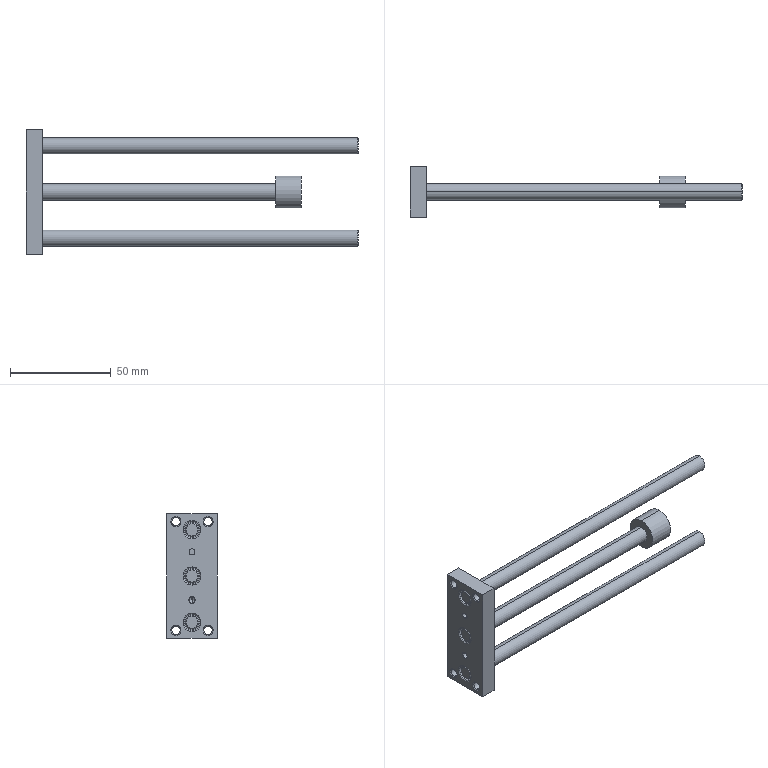Part | STEP file | _TCL-16x100-0_100fp | 1 solid | 90 faces | box 165 x 25 x 62 mm | volume 35802 mm3 | cylinder 35 | cone 34 | plane 21 | commonest cylinder face diameters 8 x12 4.134 x8 3 x7 7 x6 15.9 x2